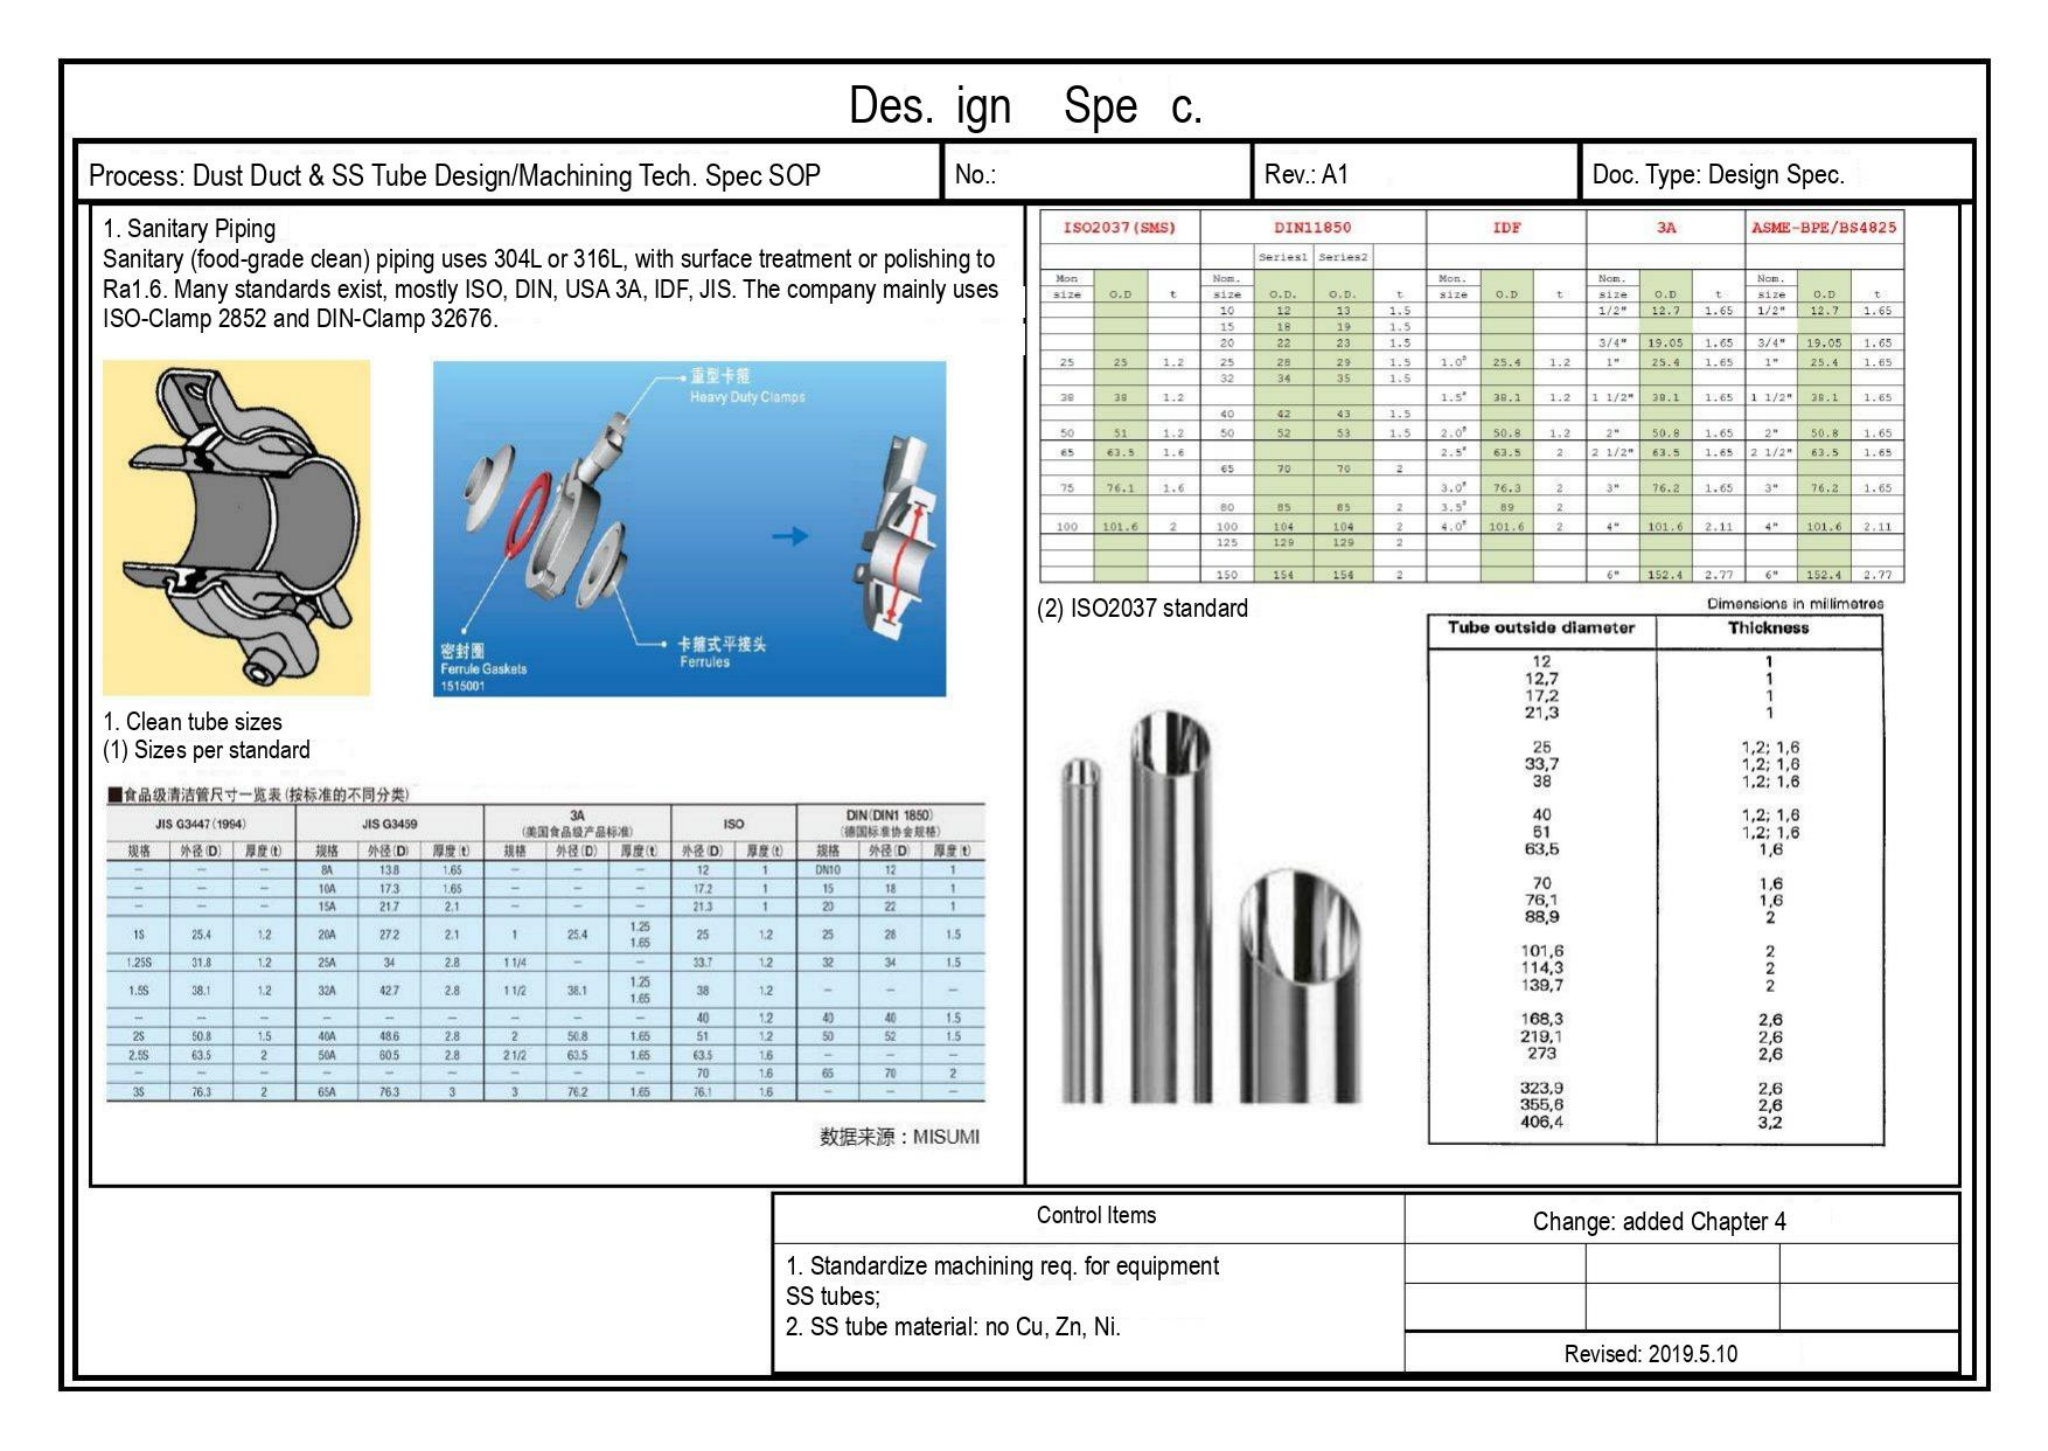Des. ign   Spe c.

| Process: Dust Duct & SS Tube Design/Machining Tech. Spec SOP | No.: | Rev.: A1 | Doc. Type: Design Spec. |
|---|---|---|---|

1. Sanitary Piping
Sanitary (food-grade clean) piping uses 304L or 316L, with surface treatment or polishing to Ra1.6. Many standards exist, mostly ISO, DIN, USA 3A, IDF, JIS. The company mainly uses ISO-Clamp 2852 and DIN-Clamp 32676.

重型卡箍
Heavy Duty Clamps

密封圈
Ferrule Gaskets
1515001

卡箍式平接头
Ferrules

1. Clean tube sizes
(1) Sizes per standard

■食品级清洁管尺寸一览表(按标准的不同分类)

| JIS G3447 (1994) 规格 | JIS G3447 (1994) 外径(D) | JIS G3447 (1994) 厚度(t) | JIS G3459 规格 | JIS G3459 外径(D) | JIS G3459 厚度(t) | 3A (美国食品级产品标准) 规格 | 3A (美国食品级产品标准) 外径(D) | 3A (美国食品级产品标准) 厚度(t) | ISO 外径(D) | ISO 厚度(t) | DIN (DIN1 1850) (德国标准协会规格) 规格 | DIN (DIN1 1850) (德国标准协会规格) 外径(D) | DIN (DIN1 1850) (德国标准协会规格) 厚度(t) |
|---|---|---|---|---|---|---|---|---|---|---|---|---|---|
| – | – | – | 8A | 13.8 | 1.65 | – | – | – | 12 | 1 | DN10 | 12 | 1 |
| – | – | – | 10A | 17.3 | 1.65 | – | – | – | 17.2 | 1 | 15 | 18 | 1 |
| – | – | – | 15A | 21.7 | 2.1 | – | – | – | 21.3 | 1 | 20 | 22 | 1 |
| 1S | 25.4 | 1.2 | 20A | 27.2 | 2.1 | 1 | 25.4 | 1.25 1.65 | 25 | 1.2 | 25 | 28 | 1.5 |
| 1.25S | 31.8 | 1.2 | 25A | 34 | 2.8 | 1 1/4 | – | – | 33.7 | 1.2 | 32 | 34 | 1.5 |
| 1.5S | 38.1 | 1.2 | 32A | 42.7 | 2.8 | 1 1/2 | 38.1 | 1.25 1.65 | 38 | 1.2 | – | – | – |
| – | – | – | – | – | – | – | – | – | 40 | 1.2 | 40 | 40 | 1.5 |
| 2S | 50.8 | 1.5 | 40A | 48.6 | 2.8 | 2 | 50.8 | 1.65 | 51 | 1.2 | 50 | 52 | 1.5 |
| 2.5S | 63.5 | 2 | 50A | 60.5 | 2.8 | 2 1/2 | 63.5 | 1.65 | 63.5 | 1.6 | – | – | – |
| – | – | – | – | – | – | – | – | – | 70 | 1.6 | 65 | 70 | 2 |
| 3S | 76.3 | 2 | 65A | 76.3 | 3 | 3 | 76.2 | 1.65 | 76.1 | 1.6 | – | – | – |

数据来源：MISUMI

| ISO2037(SMS) Mon size | ISO2037(SMS) O.D | ISO2037(SMS) t | DIN11850 Nom. size | DIN11850 Series1 O.D. | DIN11850 Series2 O.D. | DIN11850 t | IDF Mon. size | IDF O.D | IDF t | 3A Nom. size | 3A O.D | 3A t | ASME-BPE/BS4825 Nom. size | ASME-BPE/BS4825 O.D | ASME-BPE/BS4825 t |
|---|---|---|---|---|---|---|---|---|---|---|---|---|---|---|---|
| | | | 10 | 12 | 13 | 1.5 | | | | 1/2" | 12.7 | 1.65 | 1/2" | 12.7 | 1.65 |
| | | | 15 | 18 | 19 | 1.5 | | | | | | | | | |
| | | | 20 | 22 | 23 | 1.5 | | | | 3/4" | 19.05 | 1.65 | 3/4" | 19.05 | 1.65 |
| 25 | 25 | 1.2 | 25 | 28 | 29 | 1.5 | 1.0" | 25.4 | 1.2 | 1" | 25.4 | 1.65 | 1" | 25.4 | 1.65 |
| | | | 32 | 34 | 35 | 1.5 | | | | | | | | | |
| 38 | 38 | 1.2 | | | | | 1.5" | 38.1 | 1.2 | 1 1/2" | 38.1 | 1.65 | 1 1/2" | 38.1 | 1.65 |
| | | | 40 | 42 | 43 | 1.5 | | | | | | | | | |
| 50 | 51 | 1.2 | 50 | 52 | 53 | 1.5 | 2.0" | 50.8 | 1.2 | 2" | 50.8 | 1.65 | 2" | 50.8 | 1.65 |
| 65 | 63.5 | 1.6 | | | | | 2.5" | 63.5 | 2 | 2 1/2" | 63.5 | 1.65 | 2 1/2" | 63.5 | 1.65 |
| | | | 65 | 70 | 70 | 2 | | | | | | | | | |
| 75 | 76.1 | 1.6 | | | | | 3.0" | 76.3 | 2 | 3" | 76.2 | 1.65 | 3" | 76.2 | 1.65 |
| | | | 80 | 85 | 85 | 2 | 3.5" | 89 | 2 | | | | | | |
| 100 | 101.6 | 2 | 100 | 104 | 104 | 2 | 4.0" | 101.6 | 2 | 4" | 101.6 | 2.11 | 4" | 101.6 | 2.11 |
| | | | 125 | 129 | 129 | 2 | | | | | | | | | |
| | | | 150 | 154 | 154 | 2 | | | | 6" | 152.4 | 2.77 | 6" | 152.4 | 2.77 |

(2) ISO2037 standard

Dimensions in millimetres

| Tube outside diameter | Thickness |
|---|---|
| 12 | 1 |
| 12,7 | 1 |
| 17,2 | 1 |
| 21,3 | 1 |
| 25 | 1,2; 1,6 |
| 33,7 | 1,2; 1,6 |
| 38 | 1,2; 1,6 |
| 40 | 1,2; 1,6 |
| 51 | 1,2; 1,6 |
| 63,5 | 1,6 |
| 70 | 1,6 |
| 76,1 | 1,6 |
| 88,9 | 2 |
| 101,6 | 2 |
| 114,3 | 2 |
| 139,7 | 2 |
| 168,3 | 2,6 |
| 219,1 | 2,6 |
| 273 | 2,6 |
| 323,9 | 2,6 |
| 355,6 | 2,6 |
| 406,4 | 3,2 |

| Control Items | Change: added Chapter 4 |
|---|---|
| 1. Standardize machining req. for equipment SS tubes;<br>2. SS tube material: no Cu, Zn, Ni. | Revised: 2019.5.10 |
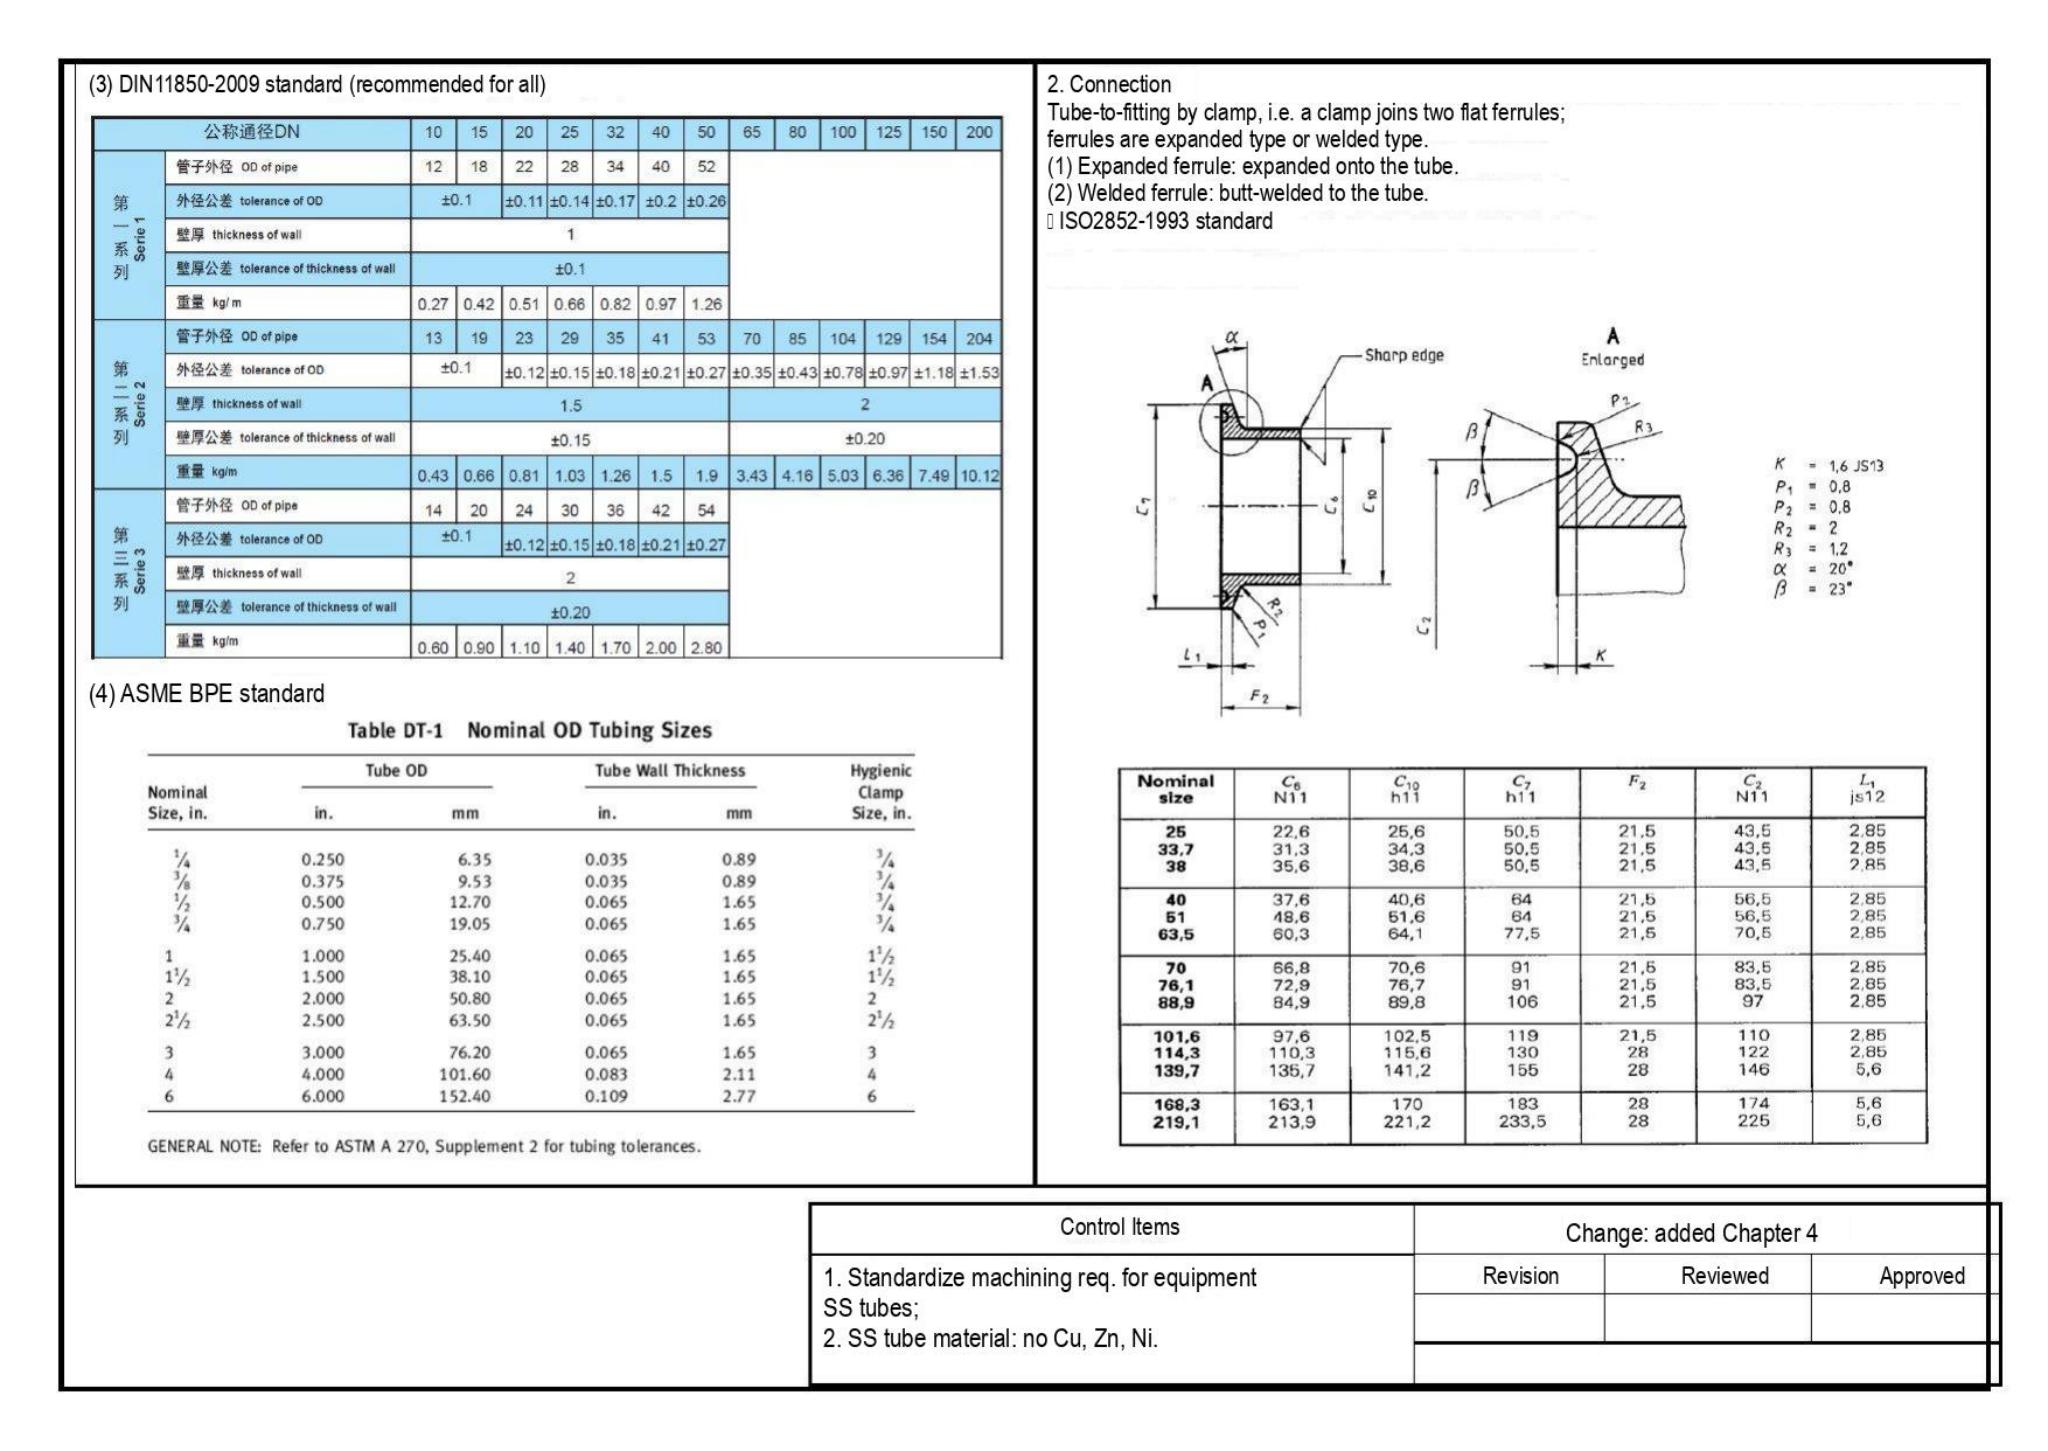(3) DIN11850-2009 standard (recommended for all)

| 公称通径DN | | 10 | 15 | 20 | 25 | 32 | 40 | 50 | 65 | 80 | 100 | 125 | 150 | 200 |
|---|---|---|---|---|---|---|---|---|---|---|---|---|---|---|
| 第一系列 Serie 1 | 管子外径 OD of pipe | 12 | 18 | 22 | 28 | 34 | 40 | 52 | | | | | | |
| | 外径公差 tolerance of OD | ±0.1 | | ±0.11 | ±0.14 | ±0.17 | ±0.2 | ±0.26 | | | | | | |
| | 壁厚 thickness of wall | 1 | | | | | | | | | | | | |
| | 壁厚公差 tolerance of thickness of wall | ±0.1 | | | | | | | | | | | | |
| | 重量 kg/ m | 0.27 | 0.42 | 0.51 | 0.66 | 0.82 | 0.97 | 1.26 | | | | | | |
| 第二系列 Serie 2 | 管子外径 OD of pipe | 13 | 19 | 23 | 29 | 35 | 41 | 53 | 70 | 85 | 104 | 129 | 154 | 204 |
| | 外径公差 tolerance of OD | ±0.1 | | ±0.12 | ±0.15 | ±0.18 | ±0.21 | ±0.27 | ±0.35 | ±0.43 | ±0.78 | ±0.97 | ±1.18 | ±1.53 |
| | 壁厚 thickness of wall | 1.5 | | | | | | | 2 | | | | | |
| | 壁厚公差 tolerance of thickness of wall | ±0.15 | | | | | | | ±0.20 | | | | | |
| | 重量 kg/m | 0.43 | 0.66 | 0.81 | 1.03 | 1.26 | 1.5 | 1.9 | 3.43 | 4.16 | 5.03 | 6.36 | 7.49 | 10.12 |
| 第三系列 Serie 3 | 管子外径 OD of pipe | 14 | 20 | 24 | 30 | 36 | 42 | 54 | | | | | | |
| | 外径公差 tolerance of OD | ±0.1 | | ±0.12 | ±0.15 | ±0.18 | ±0.21 | ±0.27 | | | | | | |
| | 壁厚 thickness of wall | 2 | | | | | | | | | | | | |
| | 壁厚公差 tolerance of thickness of wall | ±0.20 | | | | | | | | | | | | |
| | 重量 kg/m | 0.60 | 0.90 | 1.10 | 1.40 | 1.70 | 2.00 | 2.80 | | | | | | |

(4) ASME BPE standard

Table DT-1 Nominal OD Tubing Sizes

| Nominal Size, in. | Tube OD in. | Tube OD mm | Tube Wall Thickness in. | Tube Wall Thickness mm | Hygienic Clamp Size, in. |
|---|---|---|---|---|---|
| 1/4 | 0.250 | 6.35 | 0.035 | 0.89 | 3/4 |
| 3/8 | 0.375 | 9.53 | 0.035 | 0.89 | 3/4 |
| 1/2 | 0.500 | 12.70 | 0.065 | 1.65 | 3/4 |
| 3/4 | 0.750 | 19.05 | 0.065 | 1.65 | 3/4 |
| 1 | 1.000 | 25.40 | 0.065 | 1.65 | 1 1/2 |
| 1 1/2 | 1.500 | 38.10 | 0.065 | 1.65 | 1 1/2 |
| 2 | 2.000 | 50.80 | 0.065 | 1.65 | 2 |
| 2 1/2 | 2.500 | 63.50 | 0.065 | 1.65 | 2 1/2 |
| 3 | 3.000 | 76.20 | 0.065 | 1.65 | 3 |
| 4 | 4.000 | 101.60 | 0.083 | 2.11 | 4 |
| 6 | 6.000 | 152.40 | 0.109 | 2.77 | 6 |

GENERAL NOTE: Refer to ASTM A 270, Supplement 2 for tubing tolerances.

2. Connection
Tube-to-fitting by clamp, i.e. a clamp joins two flat ferrules;
ferrules are expanded type or welded type.
(1) Expanded ferrule: expanded onto the tube.
(2) Welded ferrule: butt-welded to the tube.
ISO2852-1993 standard

α
Sharp edge
A
C1
C6
C10
R2
P1
L1
F2
C2

A
Enlarged
P2
R3
β
β
K

K = 1,6 JS13
P1 = 0,8
P2 = 0,8
R2 = 2
R3 = 1,2
α = 20°
β = 23°

| Nominal size | C6 N11 | C10 h11 | C7 h11 | F2 | C2 N11 | L1 js12 |
|---|---|---|---|---|---|---|
| 25 | 22,6 | 25,6 | 50,5 | 21,5 | 43,5 | 2,85 |
| 33,7 | 31,3 | 34,3 | 50,5 | 21,5 | 43,5 | 2,85 |
| 38 | 35,6 | 38,6 | 50,5 | 21,5 | 43,5 | 2,85 |
| 40 | 37,6 | 40,6 | 64 | 21,5 | 56,5 | 2,85 |
| 51 | 48,6 | 51,6 | 64 | 21,5 | 56,5 | 2,85 |
| 63,5 | 60,3 | 64,1 | 77,5 | 21,5 | 70,5 | 2,85 |
| 70 | 66,8 | 70,6 | 91 | 21,5 | 83,5 | 2,85 |
| 76,1 | 72,9 | 76,7 | 91 | 21,5 | 83,5 | 2,85 |
| 88,9 | 84,9 | 89,8 | 106 | 21,5 | 97 | 2,85 |
| 101,6 | 97,6 | 102,5 | 119 | 21,5 | 110 | 2,85 |
| 114,3 | 110,3 | 115,6 | 130 | 28 | 122 | 2,85 |
| 139,7 | 135,7 | 141,2 | 155 | 28 | 146 | 5,6 |
| 168,3 | 163,1 | 170 | 183 | 28 | 174 | 5,6 |
| 219,1 | 213,9 | 221,2 | 233,5 | 28 | 225 | 5,6 |

| Control Items | Change: added Chapter 4 | | |
|---|---|---|---|
| 1. Standardize machining req. for equipment SS tubes;<br>2. SS tube material: no Cu, Zn, Ni. | Revision | Reviewed | Approved |
| | | | |
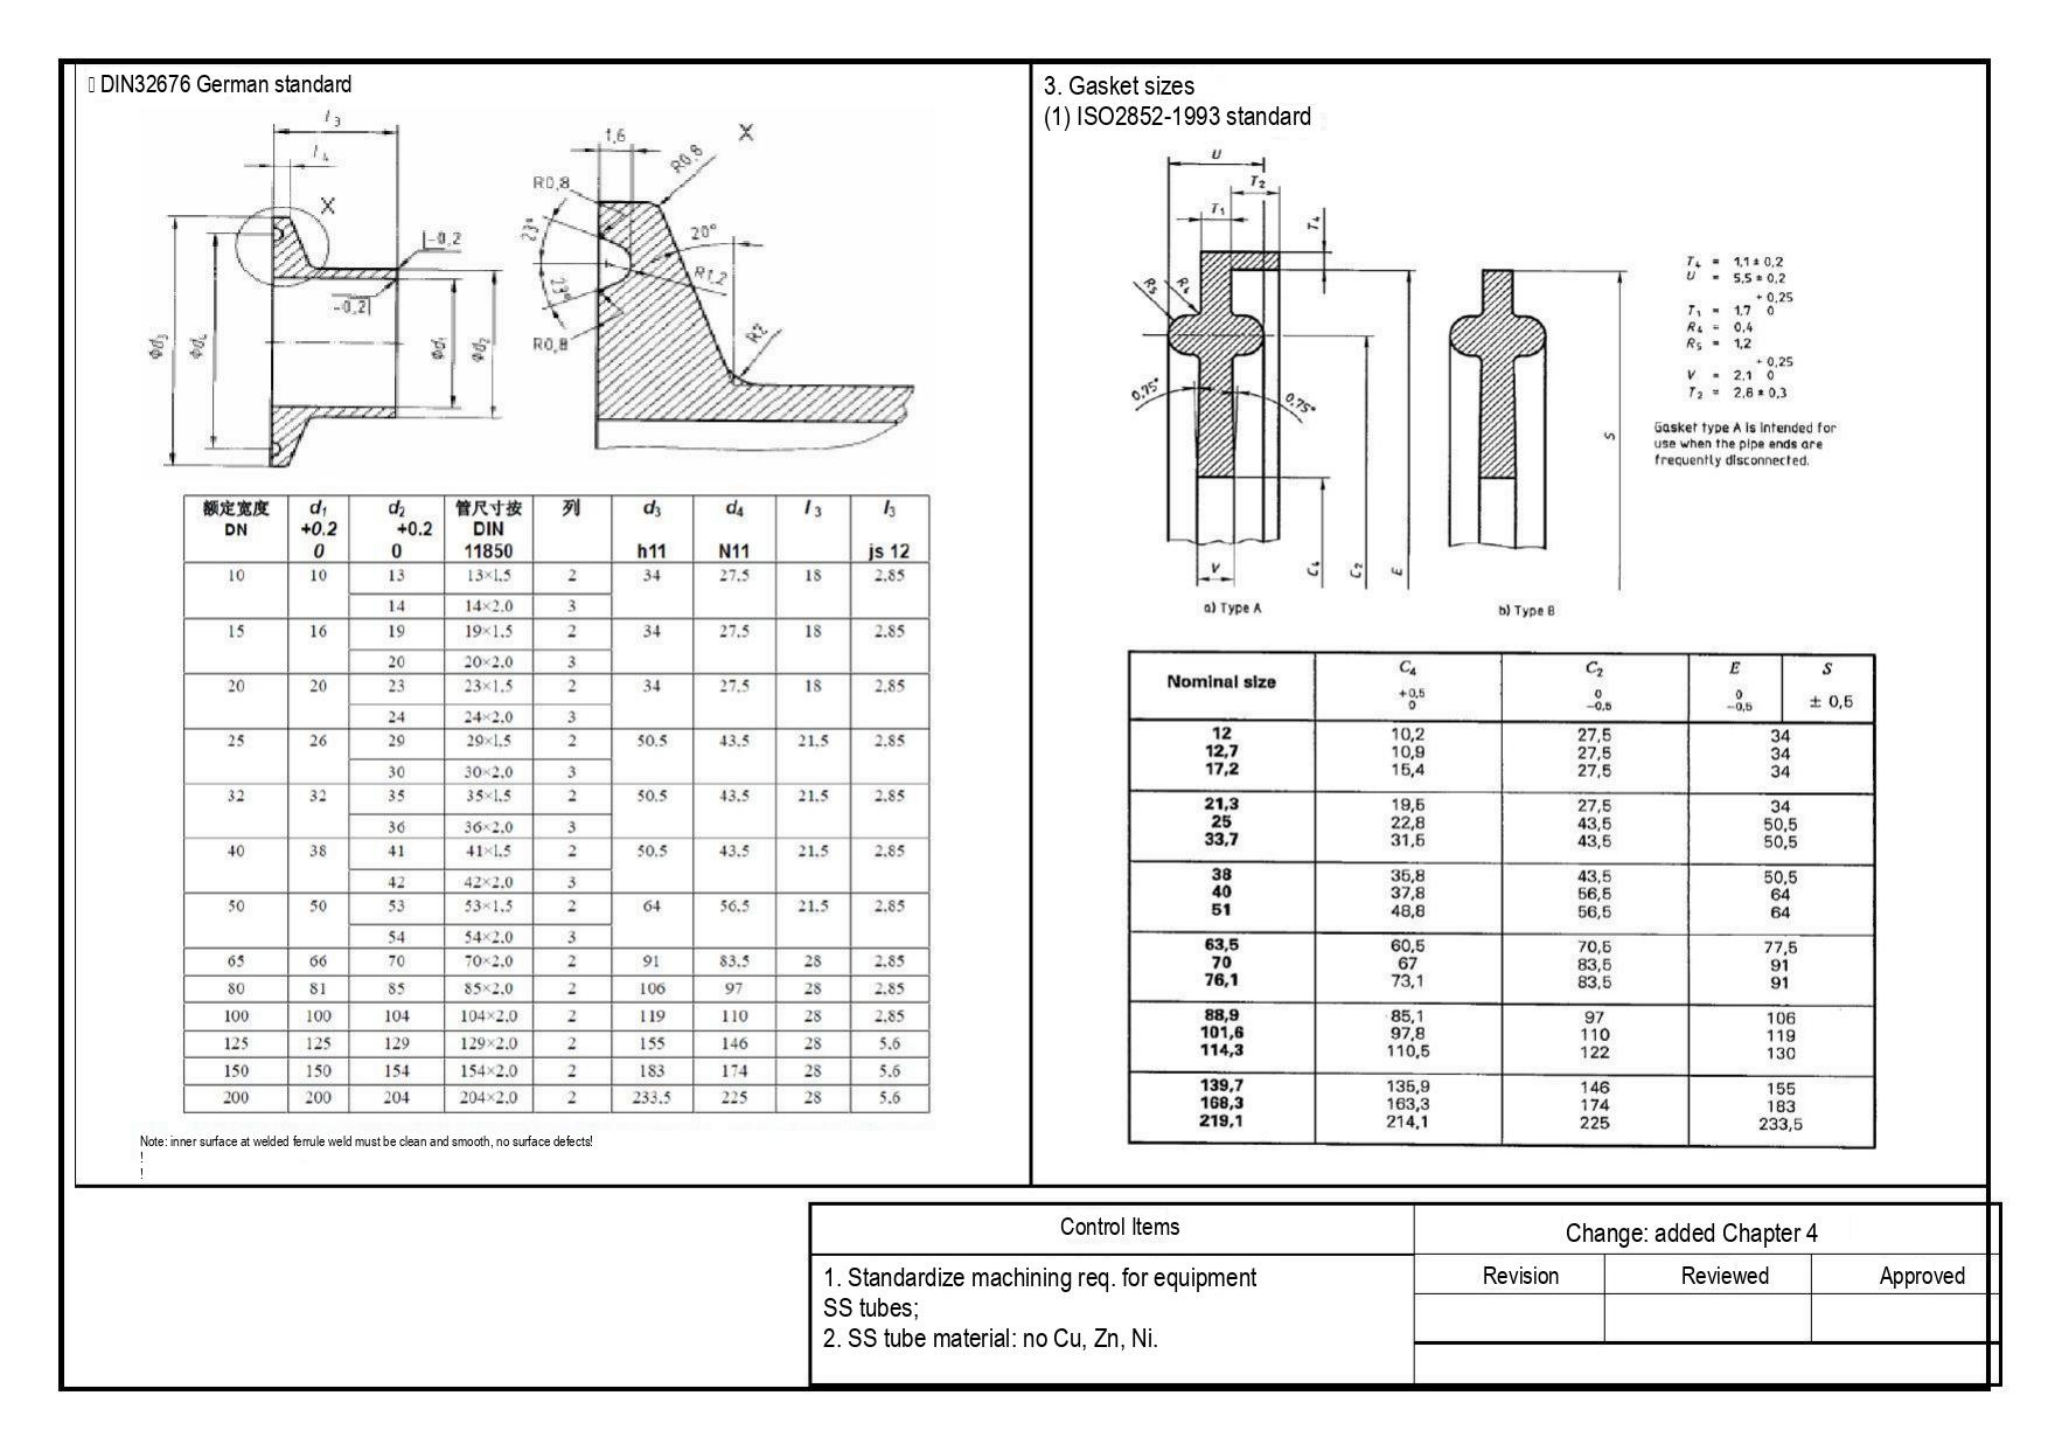DIN32676 German standard

l3
l4
X
-0,2
-0,2
Φd3
Φd4
Φd1
Φd2

1,6
R0,8
R0,8
X
23°
23°
20°
R1,2
R2
R0,8

| 额定宽度 DN | d1 +0.2 0 | d2 +0.2 0 | 管尺寸按 DIN 11850 | 列 | d3 h11 | d4 N11 | l3 | l3 js 12 |
|---|---|---|---|---|---|---|---|---|
| 10 | 10 | 13 | 13×1,5 | 2 | 34 | 27,5 | 18 | 2,85 |
| | | 14 | 14×2,0 | 3 | | | | |
| 15 | 16 | 19 | 19×1,5 | 2 | 34 | 27,5 | 18 | 2,85 |
| | | 20 | 20×2,0 | 3 | | | | |
| 20 | 20 | 23 | 23×1,5 | 2 | 34 | 27,5 | 18 | 2,85 |
| | | 24 | 24×2,0 | 3 | | | | |
| 25 | 26 | 29 | 29×1,5 | 2 | 50,5 | 43,5 | 21,5 | 2,85 |
| | | 30 | 30×2,0 | 3 | | | | |
| 32 | 32 | 35 | 35×1,5 | 2 | 50,5 | 43,5 | 21,5 | 2,85 |
| | | 36 | 36×2,0 | 3 | | | | |
| 40 | 38 | 41 | 41×1,5 | 2 | 50,5 | 43,5 | 21,5 | 2,85 |
| | | 42 | 42×2,0 | 3 | | | | |
| 50 | 50 | 53 | 53×1,5 | 2 | 64 | 56,5 | 21,5 | 2,85 |
| | | 54 | 54×2,0 | 3 | | | | |
| 65 | 66 | 70 | 70×2,0 | 2 | 91 | 83,5 | 28 | 2,85 |
| 80 | 81 | 85 | 85×2,0 | 2 | 106 | 97 | 28 | 2,85 |
| 100 | 100 | 104 | 104×2,0 | 2 | 119 | 110 | 28 | 2,85 |
| 125 | 125 | 129 | 129×2,0 | 2 | 155 | 146 | 28 | 5,6 |
| 150 | 150 | 154 | 154×2,0 | 2 | 183 | 174 | 28 | 5,6 |
| 200 | 200 | 204 | 204×2,0 | 2 | 233,5 | 225 | 28 | 5,6 |

Note: inner surface at welded ferrule weld must be clean and smooth, no surface defects!

3. Gasket sizes
(1) ISO2852-1993 standard

U
T2
T1
T4
R5
R4
0,75°
0,75°
V
C4
C2
E
S

a) Type A
b) Type B

T4 = 1,1 ± 0,2
U = 5,5 ± 0,2
T1 = 1,7 +0,25 0
R4 = 0,4
R5 = 1,2
V = 2,1 +0,25 0
T2 = 2,8 ± 0,3

Gasket type A is intended for use when the pipe ends are frequently disconnected.

| Nominal size | C4 +0,5 0 | C2 0 -0,5 | E 0 -0,5 | S ± 0,5 |
|---|---|---|---|---|
| 12<br>12,7<br>17,2 | 10,2<br>10,9<br>15,4 | 27,5<br>27,5<br>27,5 | 34<br>34<br>34 | |
| 21,3<br>25<br>33,7 | 19,6<br>22,8<br>31,6 | 27,5<br>43,5<br>43,5 | 34<br>50,5<br>50,5 | |
| 38<br>40<br>51 | 35,8<br>37,8<br>48,8 | 43,5<br>56,5<br>56,5 | 50,5<br>64<br>64 | |
| 63,5<br>70<br>76,1 | 60,5<br>67<br>73,1 | 70,5<br>83,5<br>83,5 | 77,5<br>91<br>91 | |
| 88,9<br>101,6<br>114,3 | 85,1<br>97,8<br>110,5 | 97<br>110<br>122 | 106<br>119<br>130 | |
| 139,7<br>168,3<br>219,1 | 135,9<br>163,3<br>214,1 | 146<br>174<br>225 | 155<br>183<br>233,5 | |

| Control Items | Change: added Chapter 4 | | |
|---|---|---|---|
| 1. Standardize machining req. for equipment SS tubes;<br>2. SS tube material: no Cu, Zn, Ni. | Revision | Reviewed | Approved |
| | | | |
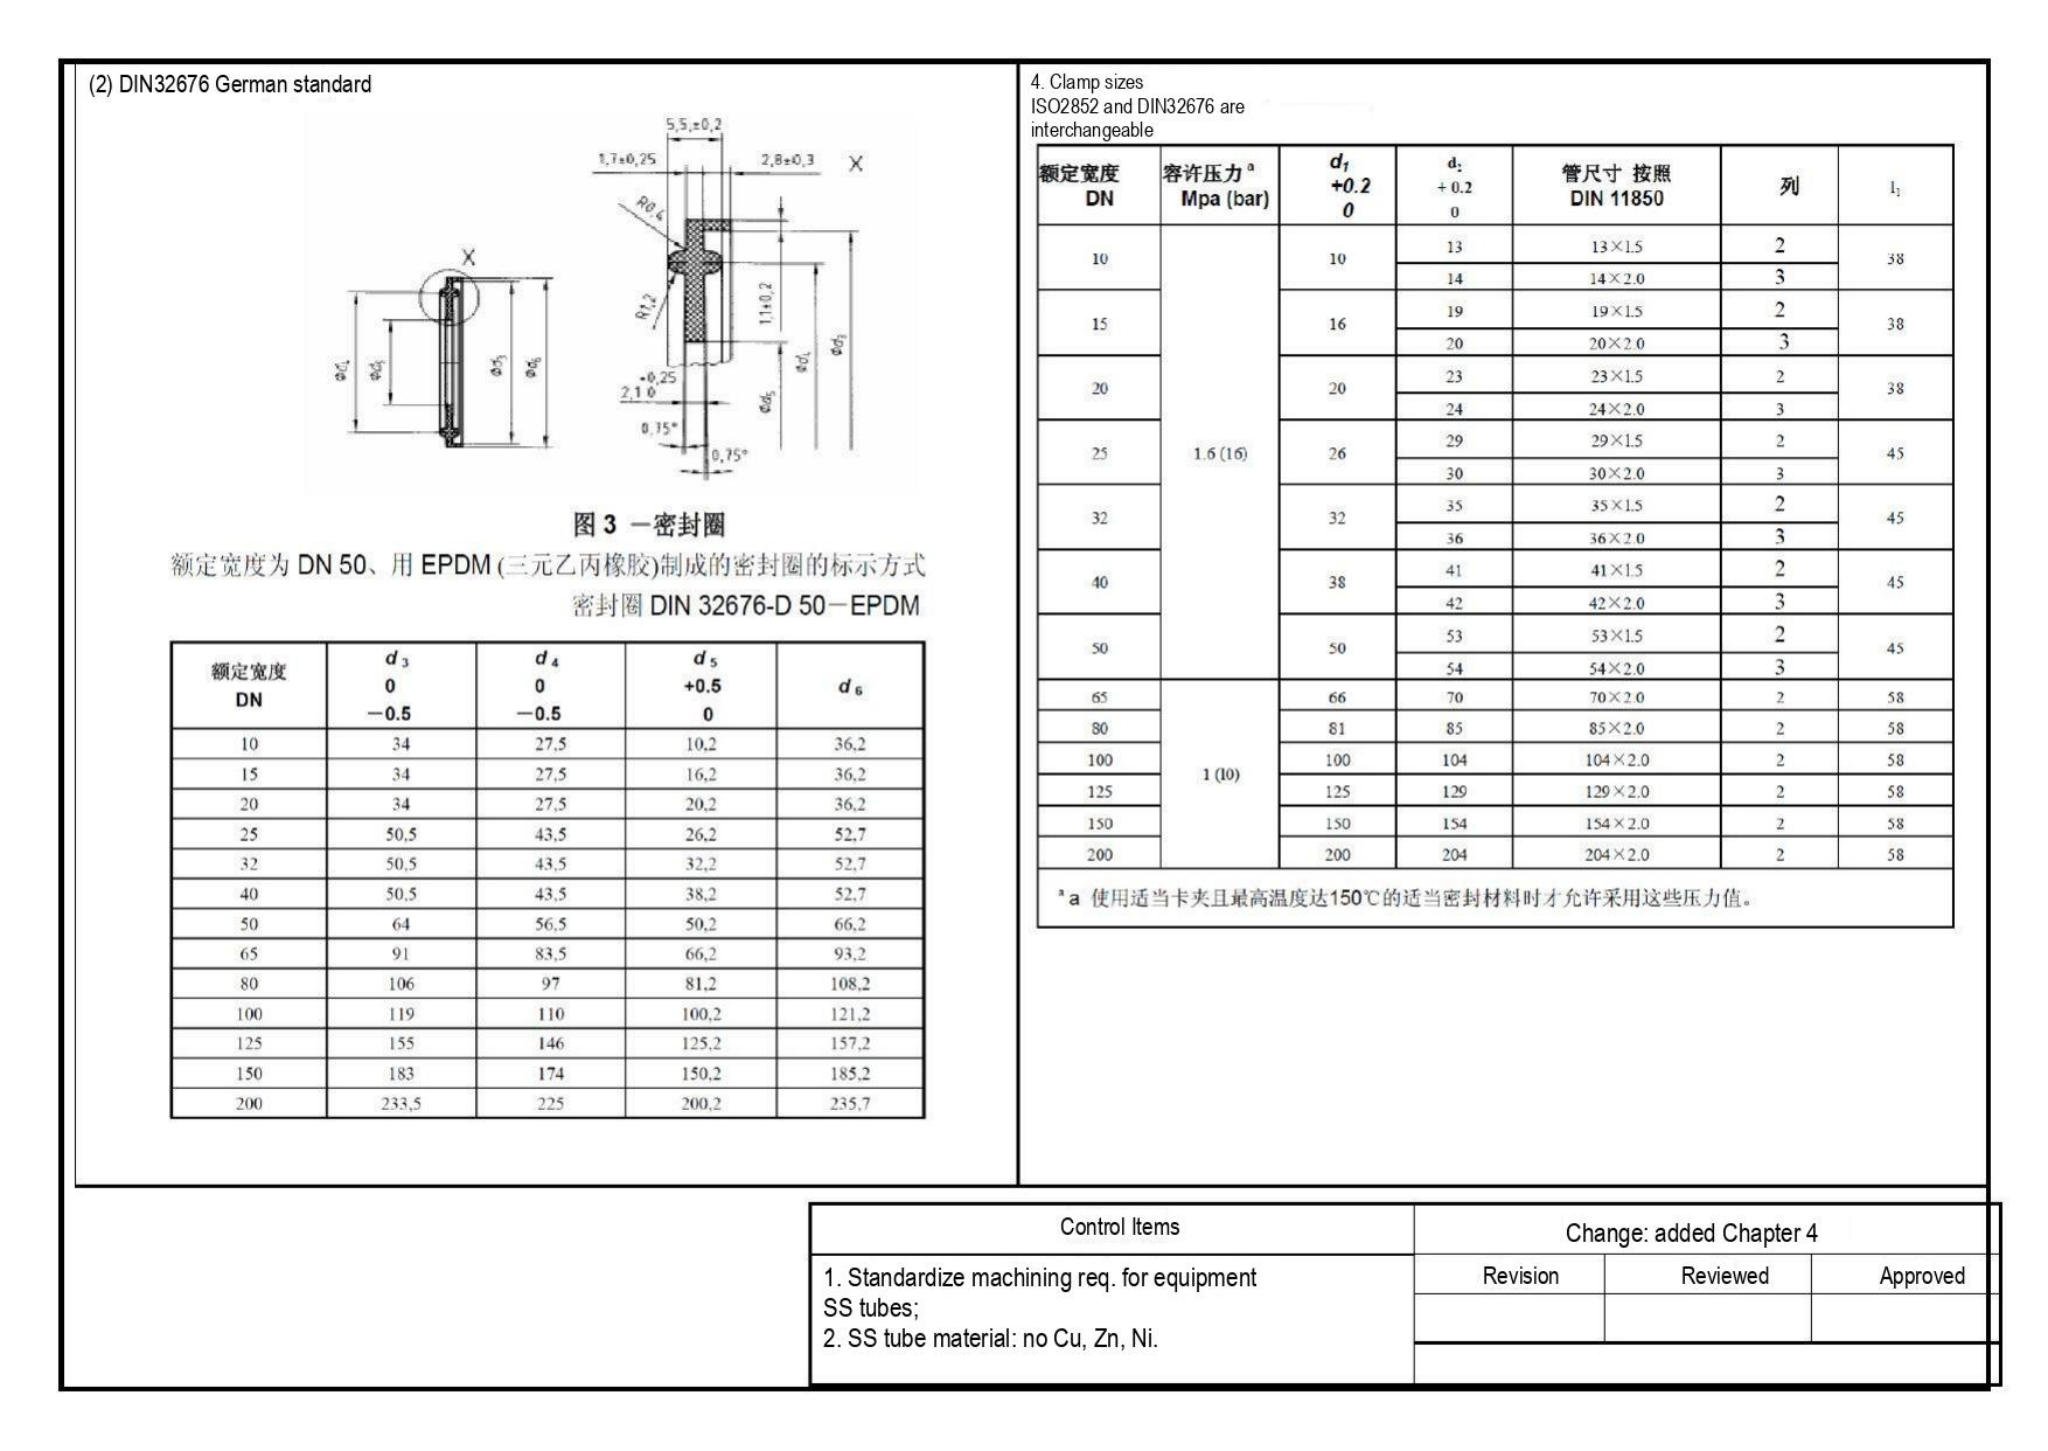(2) DIN32676 German standard

5,5±0,2
1,7±0,25
2,8±0,3
X
R0,4
X
R1,2
1,1±0,2
Ød4
Ød5
Ød6
Ød3
Ød1
Ød2
+0,25
2,1 0
0,75°
0,75°

图 3 —密封圈
额定宽度为 DN 50、用 EPDM (三元乙丙橡胶)制成的密封圈的标示方式
密封圈 DIN 32676-D 50—EPDM

| 额定宽度 DN | d₃ 0 −0.5 | d₄ 0 −0.5 | d₅ +0.5 0 | d₆ |
|---|---|---|---|---|
| 10 | 34 | 27,5 | 10,2 | 36,2 |
| 15 | 34 | 27,5 | 16,2 | 36,2 |
| 20 | 34 | 27,5 | 20,2 | 36,2 |
| 25 | 50,5 | 43,5 | 26,2 | 52,7 |
| 32 | 50,5 | 43,5 | 32,2 | 52,7 |
| 40 | 50,5 | 43,5 | 38,2 | 52,7 |
| 50 | 64 | 56,5 | 50,2 | 66,2 |
| 65 | 91 | 83,5 | 66,2 | 93,2 |
| 80 | 106 | 97 | 81,2 | 108,2 |
| 100 | 119 | 110 | 100,2 | 121,2 |
| 125 | 155 | 146 | 125,2 | 157,2 |
| 150 | 183 | 174 | 150,2 | 185,2 |
| 200 | 233,5 | 225 | 200,2 | 235,7 |

4. Clamp sizes
ISO2852 and DIN32676 are interchangeable

| 额定宽度 DN | 容许压力ᵃ Mpa (bar) | d₁ +0.2 0 | d₂ +0.2 0 | 管尺寸 按照 DIN 11850 | 列 | l₁ |
|---|---|---|---|---|---|---|
| 10 | 1.6 (16) | 10 | 13 | 13×1.5 | 2 | 38 |
| | | | 14 | 14×2.0 | 3 | |
| 15 | | 16 | 19 | 19×1.5 | 2 | 38 |
| | | | 20 | 20×2.0 | 3 | |
| 20 | | 20 | 23 | 23×1.5 | 2 | 38 |
| | | | 24 | 24×2.0 | 3 | |
| 25 | | 26 | 29 | 29×1.5 | 2 | 45 |
| | | | 30 | 30×2.0 | 3 | |
| 32 | | 32 | 35 | 35×1.5 | 2 | 45 |
| | | | 36 | 36×2.0 | 3 | |
| 40 | | 38 | 41 | 41×1.5 | 2 | 45 |
| | | | 42 | 42×2.0 | 3 | |
| 50 | | 50 | 53 | 53×1.5 | 2 | 45 |
| | | | 54 | 54×2.0 | 3 | |
| 65 | 1 (10) | 66 | 70 | 70×2.0 | 2 | 58 |
| 80 | | 81 | 85 | 85×2.0 | 2 | 58 |
| 100 | | 100 | 104 | 104×2.0 | 2 | 58 |
| 125 | | 125 | 129 | 129×2.0 | 2 | 58 |
| 150 | | 150 | 154 | 154×2.0 | 2 | 58 |
| 200 | | 200 | 204 | 204×2.0 | 2 | 58 |

ᵃa 使用适当卡夹且最高温度达150℃的适当密封材料时才允许采用这些压力值。

| Control Items | Change: added Chapter 4 | | |
|---|---|---|---|
| 1. Standardize machining req. for equipment SS tubes;<br>2. SS tube material: no Cu, Zn, Ni. | Revision | Reviewed | Approved |
| | | | |
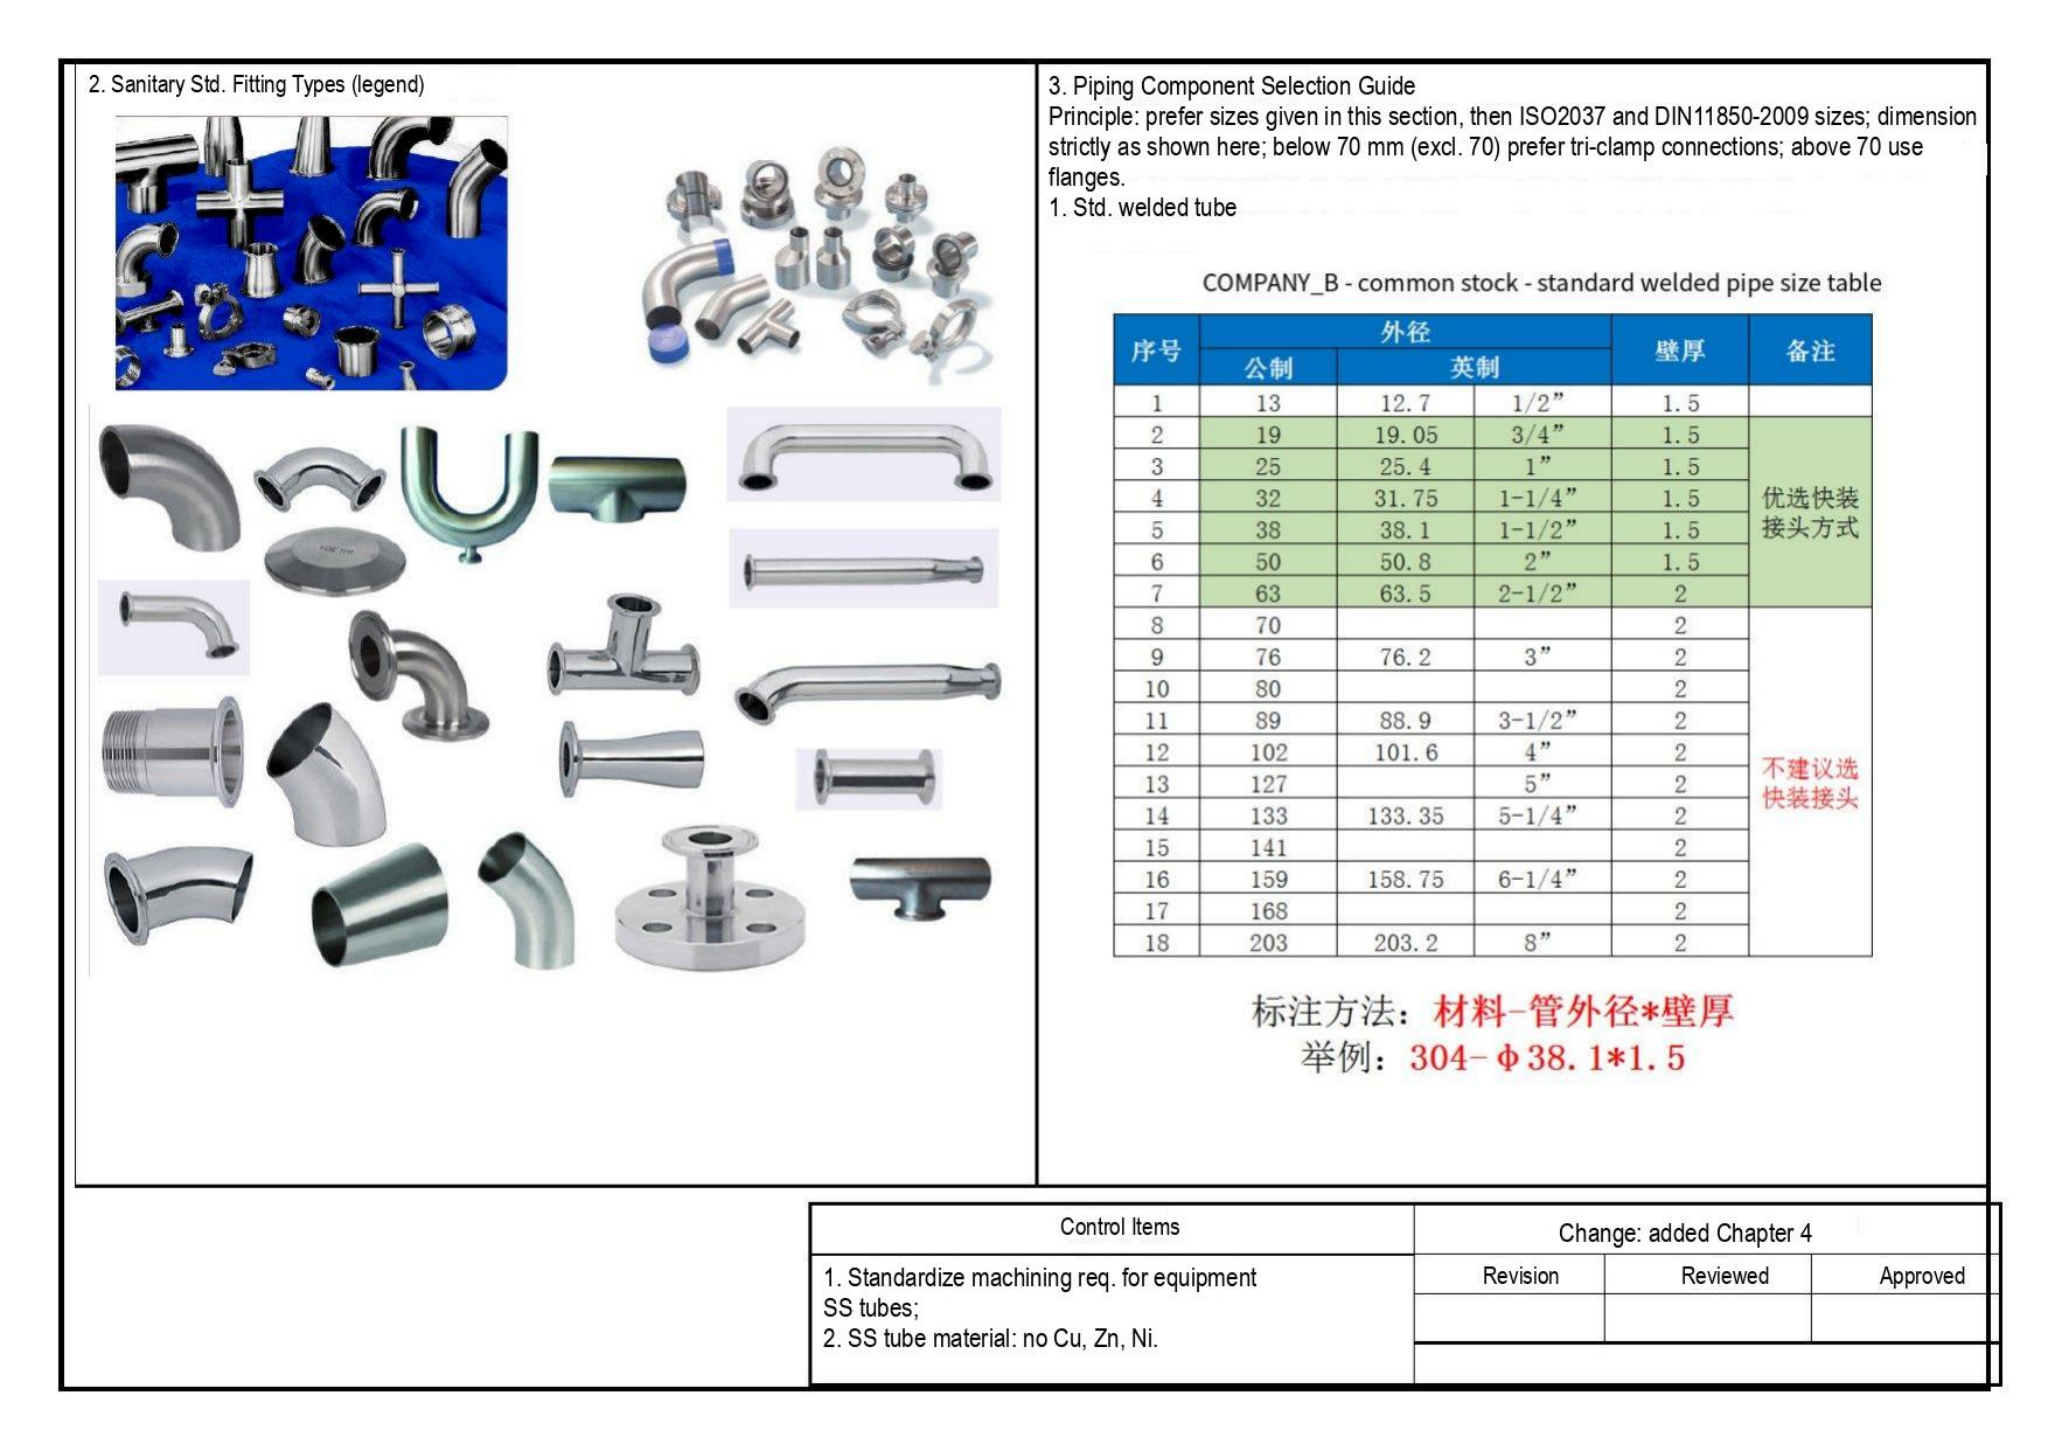2. Sanitary Std. Fitting Types (legend)

3. Piping Component Selection Guide
Principle: prefer sizes given in this section, then ISO2037 and DIN11850-2009 sizes; dimension strictly as shown here; below 70 mm (excl. 70) prefer tri-clamp connections; above 70 use flanges.
1. Std. welded tube

COMPANY_B - common stock - standard welded pipe size table

| 序号 | 外径 公制 | 外径 英制 | 外径 英制 | 壁厚 | 备注 |
|---|---|---|---|---|---|
| 1 | 13 | 12.7 | 1/2" | 1.5 | |
| 2 | 19 | 19.05 | 3/4" | 1.5 | 优选快装接头方式 |
| 3 | 25 | 25.4 | 1" | 1.5 | |
| 4 | 32 | 31.75 | 1-1/4" | 1.5 | |
| 5 | 38 | 38.1 | 1-1/2" | 1.5 | |
| 6 | 50 | 50.8 | 2" | 1.5 | |
| 7 | 63 | 63.5 | 2-1/2" | 2 | |
| 8 | 70 | | | 2 | 不建议选快装接头 |
| 9 | 76 | 76.2 | 3" | 2 | |
| 10 | 80 | | | 2 | |
| 11 | 89 | 88.9 | 3-1/2" | 2 | |
| 12 | 102 | 101.6 | 4" | 2 | |
| 13 | 127 | | 5" | 2 | |
| 14 | 133 | 133.35 | 5-1/4" | 2 | |
| 15 | 141 | | | 2 | |
| 16 | 159 | 158.75 | 6-1/4" | 2 | |
| 17 | 168 | | | 2 | |
| 18 | 203 | 203.2 | 8" | 2 | |

标注方法：材料-管外径*壁厚
举例：304-Φ38.1*1.5

| Control Items | Change: added Chapter 4 | | |
|---|---|---|---|
| 1. Standardize machining req. for equipment SS tubes;<br>2. SS tube material: no Cu, Zn, Ni. | Revision | Reviewed | Approved |
| | | | |